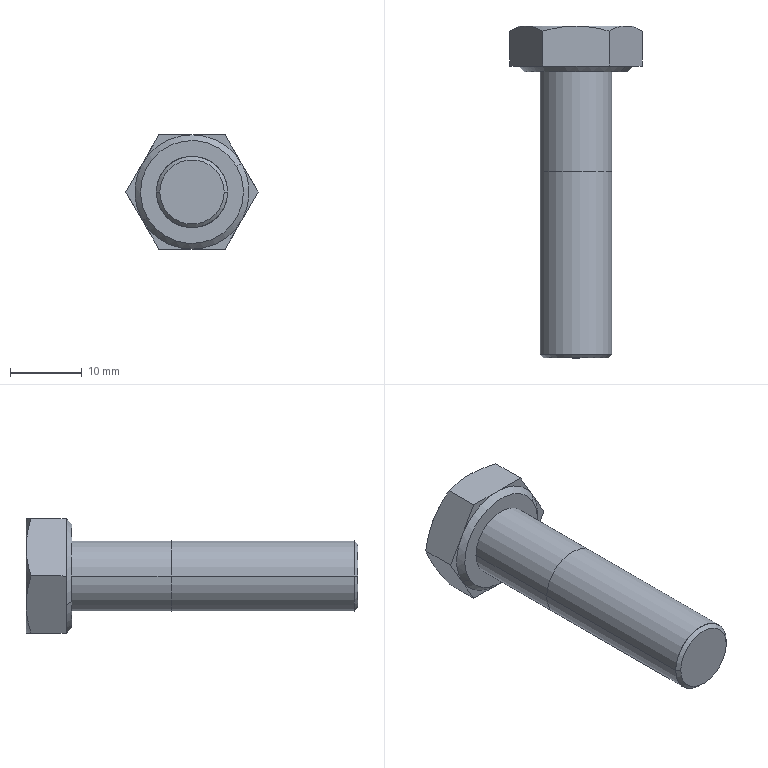Part | NX | features BREP 2 | 1 solid | 31 faces | box 18.475 x 46.4 x 16 mm | volume 5258 mm3 | plane 17 | cone 10 | cylinder 4 | commonest cylinder face diameters 8.376 x2 10 x2